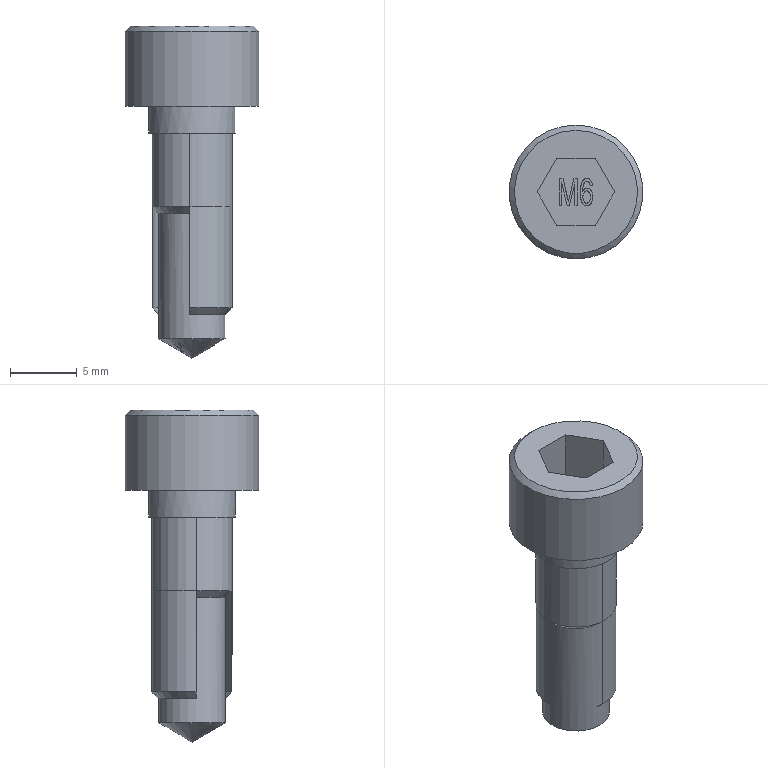Part | STEP file | M10600800 | 3 solids | 77 faces | box 10 x 10 x 24.812 mm | volume 985.086 mm3 | plane 45 | other 18 | cone 8 | cylinder 6 | commonest cylinder face diameters 6 x2 5 x1 5.98 x1 6.5 x1 10 x1